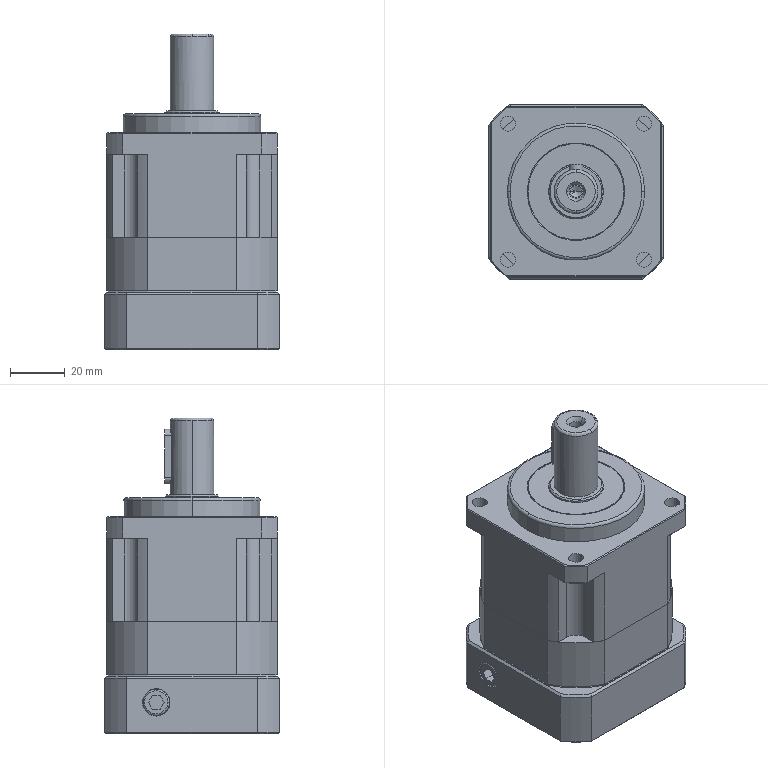Part | SolidWorks | features BaseBody 18 | 18 solids | 624 faces | box 64 x 64 x 115 mm | volume 247646 mm3 | plane 274 | cylinder 188 | cone 126 | torus 25 | spline 11 | commonest cylinder face diameters 4.2 x20 5 x20 5.5 x16 70 x12 3.3 x10 4.5 x10